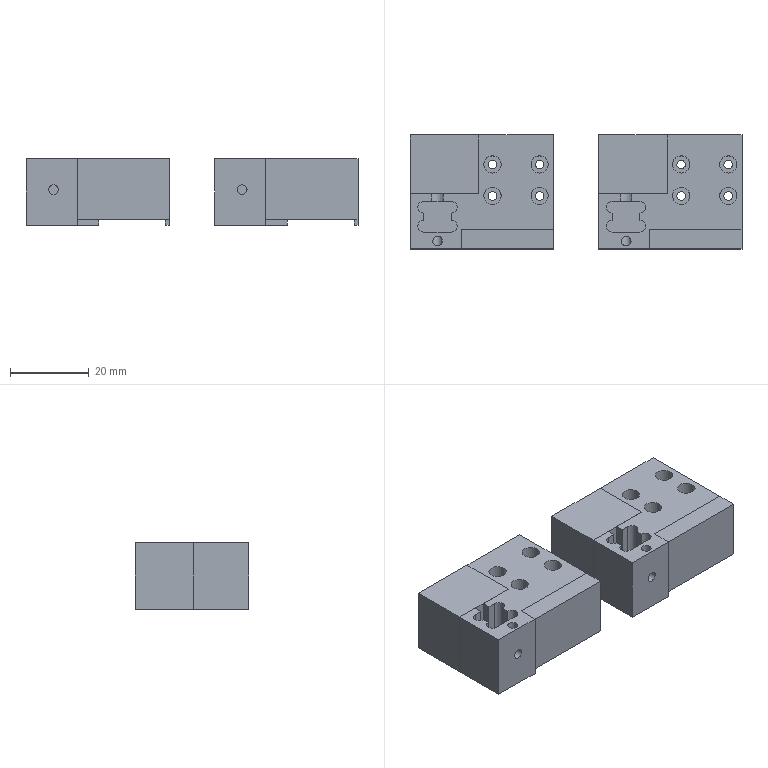NC program | NX | posted with a generic post | part box 84.5 x 29 x 17 mm
Lines 1 to 1070 of 5162:
N10 G17 G21 G94 G90
(FLOOR_WALL , TOOL : D63)
N12 T01 M6
N14 G54
N16 G17 G0 G90 X-81.75 Y0. B0. C0. S6500 M3
N18 G43 Z30. H1
N20 Z3.
N22 G94 G1 Z0. F1500.
N24 X-78.75
N26 X78.75
N28 X81.75
N30 Z3.
N32 G0 Z30.
N34 M5
(ZLEVEL_PROFILE_1 , TOOL : D10)
N36 T10 M6
N38 G54
N40 G17 G0 G90 X-39.617 Y-19.6 B0. C0. S9500 M3
N42 G43 Z30. H10
N44 Z1.5
N46 G94 G1 X-42.804 Z1.333 F1000.
N48 X-44.148 Y-19.266 Z1.26
N50 X-45.354 Y-18.584 Z1.188
N52 X-46.334 Y-17.604 Z1.115
N54 X-47.016 Y-16.398 Z1.043
N56 X-47.35 Y-15.054 Z0.97
N58 Y-14.5 Z0.941
N60 Y14.5 Z-0.579
N62 Y15.054 Z-0.608
N64 X-47.016 Y16.398 Z-0.681
N66 X-46.334 Y17.604 Z-0.753
N68 X-45.354 Y18.584 Z-0.826
N70 X-44.148 Y19.266 Z-0.898
N72 X-42.804 Y19.6 Z-0.971
N74 X-42.25 Z-1.
N76 X-5.75 F3000.
N78 G2 X-0.65 Y14.5 R5.1
N80 G1 Y-14.5
N82 G2 X-5.75 Y-19.6 R5.1
N84 G1 X-42.25
N86 G2 X-47.35 Y-14.5 R5.1
N88 G1 Y14.5
N90 G2 X-42.25 Y19.6 R5.1
N92 G1 X-5.863 Z-1.635
N94 X-5.476 Y19.593 Z-1.642
N96 X-5.091 Y19.557 Z-1.649
N98 X-4.709 Y19.493 Z-1.655
N100 X-4.334 Y19.399 Z-1.662
N102 X-3.966 Y19.278 Z-1.669
N104 X-3.609 Y19.129 Z-1.676
N106 X-3.264 Y18.953 Z-1.682
N108 X-2.934 Y18.752 Z-1.689
N110 X-2.619 Y18.526 Z-1.696
N112 X-2.323 Y18.277 Z-1.703
N114 X-2.047 Y18.006 Z-1.709
N116 X-1.791 Y17.715 Z-1.716
N118 X-1.559 Y17.406 Z-1.723
N120 X-1.351 Y17.08 Z-1.73
N122 X-1.168 Y16.739 Z-1.736
N124 X-1.011 Y16.385 Z-1.743
N126 X-0.882 Y16.02 Z-1.75
N128 X-0.781 Y15.647 Z-1.757
N130 X-0.708 Y15.266 Z-1.764
N132 X-0.664 Y14.882 Z-1.77
N134 X-0.65 Y14.495 Z-1.777
N136 Y14.108 Z-1.784
N138 Y1.721 Z-2.
N140 Y-14.5
N142 G2 X-5.75 Y-19.6 R5.1
N144 G1 X-42.25
N146 G2 X-47.35 Y-14.5 R5.1
N148 G1 Y14.5
N150 G2 X-42.25 Y19.6 R5.1
N152 G1 X-5.863 Z-2.635
N154 X-5.476 Y19.593 Z-2.642
N156 X-5.091 Y19.557 Z-2.649
N158 X-4.709 Y19.493 Z-2.655
N160 X-4.334 Y19.399 Z-2.662
N162 X-3.966 Y19.278 Z-2.669
N164 X-3.609 Y19.129 Z-2.676
N166 X-3.264 Y18.953 Z-2.682
N168 X-2.934 Y18.752 Z-2.689
N170 X-2.619 Y18.526 Z-2.696
N172 X-2.323 Y18.277 Z-2.703
N174 X-2.047 Y18.006 Z-2.709
N176 X-1.791 Y17.715 Z-2.716
N178 X-1.559 Y17.406 Z-2.723
N180 X-1.351 Y17.08 Z-2.73
N182 X-1.168 Y16.739 Z-2.736
N184 X-1.011 Y16.385 Z-2.743
N186 X-0.882 Y16.02 Z-2.75
N188 X-0.781 Y15.647 Z-2.757
N190 X-0.708 Y15.266 Z-2.764
N192 X-0.664 Y14.882 Z-2.77
N194 X-0.65 Y14.495 Z-2.777
N196 Y14.108 Z-2.784
N198 Y1.721 Z-3.
N200 Y-14.5
N202 G2 X-5.75 Y-19.6 R5.1
N204 G1 X-42.25
N206 G2 X-47.35 Y-14.5 R5.1
N208 G1 Y14.5
N210 G2 X-42.25 Y19.6 R5.1
N212 G1 X-5.863 Z-3.635
N214 X-5.476 Y19.593 Z-3.642
N216 X-5.091 Y19.557 Z-3.649
N218 X-4.709 Y19.493 Z-3.655
N220 X-4.334 Y19.399 Z-3.662
N222 X-3.966 Y19.278 Z-3.669
N224 X-3.609 Y19.129 Z-3.676
N226 X-3.264 Y18.953 Z-3.682
N228 X-2.934 Y18.752 Z-3.689
N230 X-2.619 Y18.526 Z-3.696
N232 X-2.323 Y18.277 Z-3.703
N234 X-2.047 Y18.006 Z-3.709
N236 X-1.791 Y17.715 Z-3.716
N238 X-1.559 Y17.406 Z-3.723
N240 X-1.351 Y17.08 Z-3.73
N242 X-1.168 Y16.739 Z-3.736
N244 X-1.011 Y16.385 Z-3.743
N246 X-0.882 Y16.02 Z-3.75
N248 X-0.781 Y15.647 Z-3.757
N250 X-0.708 Y15.266 Z-3.764
N252 X-0.664 Y14.882 Z-3.77
N254 X-0.65 Y14.495 Z-3.777
N256 Y14.108 Z-3.784
N258 Y1.721 Z-4.
N260 Y-14.5
N262 G2 X-5.75 Y-19.6 R5.1
N264 G1 X-42.25
N266 G2 X-47.35 Y-14.5 R5.1
N268 G1 Y14.5
N270 G2 X-42.25 Y19.6 R5.1
N272 G1 X-5.863 Z-4.635
N274 X-5.476 Y19.593 Z-4.642
N276 X-5.091 Y19.557 Z-4.649
N278 X-4.709 Y19.493 Z-4.655
N280 X-4.334 Y19.399 Z-4.662
N282 X-3.966 Y19.278 Z-4.669
N284 X-3.609 Y19.129 Z-4.676
N286 X-3.264 Y18.953 Z-4.682
N288 X-2.934 Y18.752 Z-4.689
N290 X-2.619 Y18.526 Z-4.696
N292 X-2.323 Y18.277 Z-4.703
N294 X-2.047 Y18.006 Z-4.709
N296 X-1.791 Y17.715 Z-4.716
N298 X-1.559 Y17.406 Z-4.723
N300 X-1.351 Y17.08 Z-4.73
N302 X-1.168 Y16.739 Z-4.736
N304 X-1.011 Y16.385 Z-4.743
N306 X-0.882 Y16.02 Z-4.75
N308 X-0.781 Y15.647 Z-4.757
N310 X-0.708 Y15.266 Z-4.764
N312 X-0.664 Y14.882 Z-4.77
N314 X-0.65 Y14.495 Z-4.777
N316 Y14.108 Z-4.784
N318 Y1.721 Z-5.
N320 Y-14.5
N322 G2 X-5.75 Y-19.6 R5.1
N324 G1 X-42.25
N326 G2 X-47.35 Y-14.5 R5.1
N328 G1 Y14.5
N330 G2 X-42.25 Y19.6 R5.1
N332 G1 X-5.863 Z-5.635
N334 X-5.476 Y19.593 Z-5.642
N336 X-5.091 Y19.557 Z-5.649
N338 X-4.709 Y19.493 Z-5.655
N340 X-4.334 Y19.399 Z-5.662
N342 X-3.966 Y19.278 Z-5.669
N344 X-3.609 Y19.129 Z-5.676
N346 X-3.264 Y18.953 Z-5.682
N348 X-2.934 Y18.752 Z-5.689
N350 X-2.619 Y18.526 Z-5.696
N352 X-2.323 Y18.277 Z-5.703
N354 X-2.047 Y18.006 Z-5.709
N356 X-1.791 Y17.715 Z-5.716
N358 X-1.559 Y17.406 Z-5.723
N360 X-1.351 Y17.08 Z-5.73
N362 X-1.168 Y16.739 Z-5.736
N364 X-1.011 Y16.385 Z-5.743
N366 X-0.882 Y16.02 Z-5.75
N368 X-0.781 Y15.647 Z-5.757
N370 X-0.708 Y15.266 Z-5.764
N372 X-0.664 Y14.882 Z-5.77
N374 X-0.65 Y14.495 Z-5.777
N376 Y14.108 Z-5.784
N378 Y1.721 Z-6.
N380 Y-14.5
N382 G2 X-5.75 Y-19.6 R5.1
N384 G1 X-42.25
N386 G2 X-47.35 Y-14.5 R5.1
N388 G1 Y14.5
N390 G2 X-42.25 Y19.6 R5.1
N392 G1 X-5.863 Z-6.635
N394 X-5.476 Y19.593 Z-6.642
N396 X-5.091 Y19.557 Z-6.649
N398 X-4.709 Y19.493 Z-6.655
N400 X-4.334 Y19.399 Z-6.662
N402 X-3.966 Y19.278 Z-6.669
N404 X-3.609 Y19.129 Z-6.676
N406 X-3.264 Y18.953 Z-6.682
N408 X-2.934 Y18.752 Z-6.689
N410 X-2.619 Y18.526 Z-6.696
N412 X-2.323 Y18.277 Z-6.703
N414 X-2.047 Y18.006 Z-6.709
N416 X-1.791 Y17.715 Z-6.716
N418 X-1.559 Y17.406 Z-6.723
N420 X-1.351 Y17.08 Z-6.73
N422 X-1.168 Y16.739 Z-6.736
N424 X-1.011 Y16.385 Z-6.743
N426 X-0.882 Y16.02 Z-6.75
N428 X-0.781 Y15.647 Z-6.757
N430 X-0.708 Y15.266 Z-6.764
N432 X-0.664 Y14.882 Z-6.77
N434 X-0.65 Y14.495 Z-6.777
N436 Y14.108 Z-6.784
N438 Y1.721 Z-7.
N440 Y-14.5
N442 G2 X-5.75 Y-19.6 R5.1
N444 G1 X-42.25
N446 G2 X-47.35 Y-14.5 R5.1
N448 G1 Y14.5
N450 G2 X-42.25 Y19.6 R5.1
N452 G1 X-5.863 Z-7.635
N454 X-5.476 Y19.593 Z-7.642
N456 X-5.091 Y19.557 Z-7.649
N458 X-4.709 Y19.493 Z-7.655
N460 X-4.334 Y19.399 Z-7.662
N462 X-3.966 Y19.278 Z-7.669
N464 X-3.609 Y19.129 Z-7.676
N466 X-3.264 Y18.953 Z-7.682
N468 X-2.934 Y18.752 Z-7.689
N470 X-2.619 Y18.526 Z-7.696
N472 X-2.323 Y18.277 Z-7.703
N474 X-2.047 Y18.006 Z-7.709
N476 X-1.791 Y17.715 Z-7.716
N478 X-1.559 Y17.406 Z-7.723
N480 X-1.351 Y17.08 Z-7.73
N482 X-1.168 Y16.739 Z-7.736
N484 X-1.011 Y16.385 Z-7.743
N486 X-0.882 Y16.02 Z-7.75
N488 X-0.781 Y15.647 Z-7.757
N490 X-0.708 Y15.266 Z-7.764
N492 X-0.664 Y14.882 Z-7.77
N494 X-0.65 Y14.495 Z-7.777
N496 Y14.108 Z-7.784
N498 Y1.721 Z-8.
N500 Y-14.5
N502 G2 X-5.75 Y-19.6 R5.1
N504 G1 X-42.25
N506 G2 X-47.35 Y-14.5 R5.1
N508 G1 Y14.5
N510 G2 X-42.25 Y19.6 R5.1
N512 G1 X-5.863 Z-8.635
N514 X-5.476 Y19.593 Z-8.642
N516 X-5.091 Y19.557 Z-8.649
N518 X-4.709 Y19.493 Z-8.655
N520 X-4.334 Y19.399 Z-8.662
N522 X-3.966 Y19.278 Z-8.669
N524 X-3.609 Y19.129 Z-8.676
N526 X-3.264 Y18.953 Z-8.682
N528 X-2.934 Y18.752 Z-8.689
N530 X-2.619 Y18.526 Z-8.696
N532 X-2.323 Y18.277 Z-8.703
N534 X-2.047 Y18.006 Z-8.709
N536 X-1.791 Y17.715 Z-8.716
N538 X-1.559 Y17.406 Z-8.723
N540 X-1.351 Y17.08 Z-8.73
N542 X-1.168 Y16.739 Z-8.736
N544 X-1.011 Y16.385 Z-8.743
N546 X-0.882 Y16.02 Z-8.75
N548 X-0.781 Y15.647 Z-8.757
N550 X-0.708 Y15.266 Z-8.764
N552 X-0.664 Y14.882 Z-8.77
N554 X-0.65 Y14.495 Z-8.777
N556 Y14.108 Z-8.784
N558 Y1.721 Z-9.
N560 Y-14.5
N562 G2 X-5.75 Y-19.6 R5.1
N564 G1 X-42.25
N566 G2 X-47.35 Y-14.5 R5.1
N568 G1 Y14.5
N570 G2 X-42.25 Y19.6 R5.1
N572 G1 X-5.863 Z-9.635
N574 X-5.476 Y19.593 Z-9.642
N576 X-5.091 Y19.557 Z-9.649
N578 X-4.709 Y19.493 Z-9.655
N580 X-4.334 Y19.399 Z-9.662
N582 X-3.966 Y19.278 Z-9.669
N584 X-3.609 Y19.129 Z-9.676
N586 X-3.264 Y18.953 Z-9.682
N588 X-2.934 Y18.752 Z-9.689
N590 X-2.619 Y18.526 Z-9.696
N592 X-2.323 Y18.277 Z-9.703
N594 X-2.047 Y18.006 Z-9.709
N596 X-1.791 Y17.715 Z-9.716
N598 X-1.559 Y17.406 Z-9.723
N600 X-1.351 Y17.08 Z-9.73
N602 X-1.168 Y16.739 Z-9.736
N604 X-1.011 Y16.385 Z-9.743
N606 X-0.882 Y16.02 Z-9.75
N608 X-0.781 Y15.647 Z-9.757
N610 X-0.708 Y15.266 Z-9.764
N612 X-0.664 Y14.882 Z-9.77
N614 X-0.65 Y14.495 Z-9.777
N616 Y14.108 Z-9.784
N618 Y1.721 Z-10.
N620 Y-14.5
N622 G2 X-5.75 Y-19.6 R5.1
N624 G1 X-42.25
N626 G2 X-47.35 Y-14.5 R5.1
N628 G1 Y14.5
N630 G2 X-42.25 Y19.6 R5.1
N632 G1 X-5.863 Z-10.635
N634 X-5.476 Y19.593 Z-10.642
N636 X-5.091 Y19.557 Z-10.649
N638 X-4.709 Y19.493 Z-10.655
N640 X-4.334 Y19.399 Z-10.662
N642 X-3.966 Y19.278 Z-10.669
N644 X-3.609 Y19.129 Z-10.676
N646 X-3.264 Y18.953 Z-10.682
N648 X-2.934 Y18.752 Z-10.689
N650 X-2.619 Y18.526 Z-10.696
N652 X-2.323 Y18.277 Z-10.703
N654 X-2.047 Y18.006 Z-10.709
N656 X-1.791 Y17.715 Z-10.716
N658 X-1.559 Y17.406 Z-10.723
N660 X-1.351 Y17.08 Z-10.73
N662 X-1.168 Y16.739 Z-10.736
N664 X-1.011 Y16.385 Z-10.743
N666 X-0.882 Y16.02 Z-10.75
N668 X-0.781 Y15.647 Z-10.757
N670 X-0.708 Y15.266 Z-10.764
N672 X-0.664 Y14.882 Z-10.77
N674 X-0.65 Y14.495 Z-10.777
N676 Y14.108 Z-10.784
N678 Y1.721 Z-11.
N680 Y-14.5
N682 G2 X-5.75 Y-19.6 R5.1
N684 G1 X-42.25
N686 G2 X-47.35 Y-14.5 R5.1
N688 G1 Y14.5
N690 G2 X-42.25 Y19.6 R5.1
N692 G1 X-5.863 Z-11.635
N694 X-5.476 Y19.593 Z-11.642
N696 X-5.091 Y19.557 Z-11.649
N698 X-4.709 Y19.493 Z-11.655
N700 X-4.334 Y19.399 Z-11.662
N702 X-3.966 Y19.278 Z-11.669
N704 X-3.609 Y19.129 Z-11.676
N706 X-3.264 Y18.953 Z-11.682
N708 X-2.934 Y18.752 Z-11.689
N710 X-2.619 Y18.526 Z-11.696
N712 X-2.323 Y18.277 Z-11.703
N714 X-2.047 Y18.006 Z-11.709
N716 X-1.791 Y17.715 Z-11.716
N718 X-1.559 Y17.406 Z-11.723
N720 X-1.351 Y17.08 Z-11.73
N722 X-1.168 Y16.739 Z-11.736
N724 X-1.011 Y16.385 Z-11.743
N726 X-0.882 Y16.02 Z-11.75
N728 X-0.781 Y15.647 Z-11.757
N730 X-0.708 Y15.266 Z-11.764
N732 X-0.664 Y14.882 Z-11.77
N734 X-0.65 Y14.495 Z-11.777
N736 Y14.108 Z-11.784
N738 Y1.721 Z-12.
N740 Y-14.5
N742 G2 X-5.75 Y-19.6 R5.1
N744 G1 X-42.25
N746 G2 X-47.35 Y-14.5 R5.1
N748 G1 Y14.5
N750 G2 X-42.25 Y19.6 R5.1
N752 G1 X-5.863 Z-12.635
N754 X-5.476 Y19.593 Z-12.642
N756 X-5.091 Y19.557 Z-12.649
N758 X-4.709 Y19.493 Z-12.655
N760 X-4.334 Y19.399 Z-12.662
N762 X-3.966 Y19.278 Z-12.669
N764 X-3.609 Y19.129 Z-12.676
N766 X-3.264 Y18.953 Z-12.682
N768 X-2.934 Y18.752 Z-12.689
N770 X-2.619 Y18.526 Z-12.696
N772 X-2.323 Y18.277 Z-12.703
N774 X-2.047 Y18.006 Z-12.709
N776 X-1.791 Y17.715 Z-12.716
N778 X-1.559 Y17.406 Z-12.723
N780 X-1.351 Y17.08 Z-12.73
N782 X-1.168 Y16.739 Z-12.736
N784 X-1.011 Y16.385 Z-12.743
N786 X-0.882 Y16.02 Z-12.75
N788 X-0.781 Y15.647 Z-12.757
N790 X-0.708 Y15.266 Z-12.764
N792 X-0.664 Y14.882 Z-12.77
N794 X-0.65 Y14.495 Z-12.777
N796 Y14.108 Z-12.784
N798 Y1.721 Z-13.
N800 Y-14.5
N802 G2 X-5.75 Y-19.6 R5.1
N804 G1 X-42.25
N806 G2 X-47.35 Y-14.5 R5.1
N808 G1 Y14.5
N810 G2 X-42.25 Y19.6 R5.1
N812 G1 X-5.863 Z-13.635
N814 X-5.476 Y19.593 Z-13.642
N816 X-5.091 Y19.557 Z-13.649
N818 X-4.709 Y19.493 Z-13.655
N820 X-4.334 Y19.399 Z-13.662
N822 X-3.966 Y19.278 Z-13.669
N824 X-3.609 Y19.129 Z-13.676
N826 X-3.264 Y18.953 Z-13.682
N828 X-2.934 Y18.752 Z-13.689
N830 X-2.619 Y18.526 Z-13.696
N832 X-2.323 Y18.277 Z-13.703
N834 X-2.047 Y18.006 Z-13.709
N836 X-1.791 Y17.715 Z-13.716
N838 X-1.559 Y17.406 Z-13.723
N840 X-1.351 Y17.08 Z-13.73
N842 X-1.168 Y16.739 Z-13.736
N844 X-1.011 Y16.385 Z-13.743
N846 X-0.882 Y16.02 Z-13.75
N848 X-0.781 Y15.647 Z-13.757
N850 X-0.708 Y15.266 Z-13.764
N852 X-0.664 Y14.882 Z-13.77
N854 X-0.65 Y14.495 Z-13.777
N856 Y14.108 Z-13.784
N858 Y1.721 Z-14.
N860 Y-14.5
N862 G2 X-5.75 Y-19.6 R5.1
N864 G1 X-42.25
N866 G2 X-47.35 Y-14.5 R5.1
N868 G1 Y14.5
N870 G2 X-42.25 Y19.6 R5.1
N872 G1 X-5.863 Z-14.635
N874 X-5.476 Y19.593 Z-14.642
N876 X-5.091 Y19.557 Z-14.649
N878 X-4.709 Y19.493 Z-14.655
N880 X-4.334 Y19.399 Z-14.662
N882 X-3.966 Y19.278 Z-14.669
N884 X-3.609 Y19.129 Z-14.676
N886 X-3.264 Y18.953 Z-14.682
N888 X-2.934 Y18.752 Z-14.689
N890 X-2.619 Y18.526 Z-14.696
N892 X-2.323 Y18.277 Z-14.703
N894 X-2.047 Y18.006 Z-14.709
N896 X-1.791 Y17.715 Z-14.716
N898 X-1.559 Y17.406 Z-14.723
N900 X-1.351 Y17.08 Z-14.73
N902 X-1.168 Y16.739 Z-14.736
N904 X-1.011 Y16.385 Z-14.743
N906 X-0.882 Y16.02 Z-14.75
N908 X-0.781 Y15.647 Z-14.757
N910 X-0.708 Y15.266 Z-14.764
N912 X-0.664 Y14.882 Z-14.77
N914 X-0.65 Y14.495 Z-14.777
N916 Y14.108 Z-14.784
N918 Y1.721 Z-15.
N920 Y-14.5
N922 G2 X-5.75 Y-19.6 R5.1
N924 G1 X-42.25
N926 G2 X-47.35 Y-14.5 R5.1
N928 G1 Y14.5
N930 G2 X-42.25 Y19.6 R5.1
N932 G1 X-5.863 Z-15.635
N934 X-5.476 Y19.593 Z-15.642
N936 X-5.091 Y19.557 Z-15.649
N938 X-4.709 Y19.493 Z-15.655
N940 X-4.334 Y19.399 Z-15.662
N942 X-3.966 Y19.278 Z-15.669
N944 X-3.609 Y19.129 Z-15.676
N946 X-3.264 Y18.953 Z-15.682
N948 X-2.934 Y18.752 Z-15.689
N950 X-2.619 Y18.526 Z-15.696
N952 X-2.323 Y18.277 Z-15.703
N954 X-2.047 Y18.006 Z-15.709
N956 X-1.791 Y17.715 Z-15.716
N958 X-1.559 Y17.406 Z-15.723
N960 X-1.351 Y17.08 Z-15.73
N962 X-1.168 Y16.739 Z-15.736
N964 X-1.011 Y16.385 Z-15.743
N966 X-0.882 Y16.02 Z-15.75
N968 X-0.781 Y15.647 Z-15.757
N970 X-0.708 Y15.266 Z-15.764
N972 X-0.664 Y14.882 Z-15.77
N974 X-0.65 Y14.495 Z-15.777
N976 Y14.108 Z-15.784
N978 Y1.721 Z-16.
N980 Y-14.5
N982 G2 X-5.75 Y-19.6 R5.1
N984 G1 X-42.25
N986 G2 X-47.35 Y-14.5 R5.1
N988 G1 Y14.5
N990 G2 X-42.25 Y19.6 R5.1
N992 G1 X-5.863 Z-16.635
N994 X-5.476 Y19.593 Z-16.642
N996 X-5.091 Y19.557 Z-16.649
N998 X-4.709 Y19.493 Z-16.655
N1000 X-4.334 Y19.399 Z-16.662
N1002 X-3.966 Y19.278 Z-16.669
N1004 X-3.609 Y19.129 Z-16.676
N1006 X-3.264 Y18.953 Z-16.682
N1008 X-2.934 Y18.752 Z-16.689
N1010 X-2.619 Y18.526 Z-16.696
N1012 X-2.323 Y18.277 Z-16.703
N1014 X-2.047 Y18.006 Z-16.709
N1016 X-1.791 Y17.715 Z-16.716
N1018 X-1.559 Y17.406 Z-16.723
N1020 X-1.351 Y17.08 Z-16.73
N1022 X-1.168 Y16.739 Z-16.736
N1024 X-1.011 Y16.385 Z-16.743
N1026 X-0.882 Y16.02 Z-16.75
N1028 X-0.781 Y15.647 Z-16.757
N1030 X-0.708 Y15.266 Z-16.764
N1032 X-0.664 Y14.882 Z-16.77
N1034 X-0.65 Y14.495 Z-16.777
N1036 Y14.108 Z-16.784
N1038 Y1.721 Z-17.
N1040 Y-14.5
N1042 G2 X-5.75 Y-19.6 R5.1
N1044 G1 X-42.25
N1046 G2 X-47.35 Y-14.5 R5.1
N1048 G1 Y14.5
N1050 G2 X-42.25 Y19.6 R5.1
N1052 G1 X-5.75
N1054 G2 X-0.65 Y14.5 R5.1
N1056 G1 Y1.721
N1058 Z-15.5
N1060 G0 Z30.
N1062 X8.383 Y-19.6
N1064 Z1.5
N1066 G1 X5.196 Z1.333 F1000.
N1068 X3.852 Y-19.266 Z1.26
N1070 X2.646 Y-18.584 Z1.188
N1072 X1.666 Y-17.604 Z1.115
N1074 X0.984 Y-16.398 Z1.043
N1076 X0.65 Y-15.054 Z0.97
N1078 Y15.054 Z-0.608
N1080 X0.984 Y16.398 Z-0.681
N1082 X1.666 Y17.604 Z-0.753
N1084 X2.646 Y18.584 Z-0.826
N1086 X3.852 Y19.266 Z-0.898
N1088 X5.196 Y19.6 Z-0.971
N1090 X5.75 Z-1.
N1092 X42.25 F3000.
N1094 G2 X47.35 Y14.5 R5.1
N1096 G1 Y-14.5
N1098 G2 X42.25 Y-19.6 R5.1
N1100 G1 X5.75
N1102 G2 X0.65 Y-14.5 R5.1
N1104 G1 Y14.5
N1106 G2 X5.75 Y19.6 R5.1
N1108 G1 X42.137 Z-1.635
N1110 X42.524 Y19.593 Z-1.642
N1112 X42.909 Y19.557 Z-1.649
N1114 X43.291 Y19.493 Z-1.655
N1116 X43.666 Y19.399 Z-1.662
N1118 X44.034 Y19.278 Z-1.669
N1120 X44.391 Y19.129 Z-1.676
N1122 X44.736 Y18.953 Z-1.682
N1124 X45.066 Y18.752 Z-1.689
N1126 X45.381 Y18.526 Z-1.696
N1128 X45.677 Y18.277 Z-1.703
N1130 X45.953 Y18.006 Z-1.709
N1132 X46.209 Y17.715 Z-1.716
N1134 X46.441 Y17.406 Z-1.723
N1136 X46.649 Y17.08 Z-1.73
N1138 X46.832 Y16.739 Z-1.736
N1140 X46.989 Y16.385 Z-1.743
N1142 X47.118 Y16.02 Z-1.75
N1144 X47.219 Y15.647 Z-1.757
N1146 X47.292 Y15.266 Z-1.764
N1148 X47.336 Y14.882 Z-1.77
N1150 X47.35 Y14.495 Z-1.777
N1152 Y14.108 Z-1.784
N1154 Y1.721 Z-2.
N1156 Y-14.5
N1158 G2 X42.25 Y-19.6 R5.1
N1160 G1 X5.75
N1162 G2 X0.65 Y-14.5 R5.1
N1164 G1 Y14.5
N1166 G2 X5.75 Y19.6 R5.1
N1168 G1 X42.137 Z-2.635
N1170 X42.524 Y19.593 Z-2.642
N1172 X42.909 Y19.557 Z-2.649
N1174 X43.291 Y19.493 Z-2.655
N1176 X43.666 Y19.399 Z-2.662
N1178 X44.034 Y19.278 Z-2.669
N1180 X44.391 Y19.129 Z-2.676
N1182 X44.736 Y18.953 Z-2.682
N1184 X45.066 Y18.752 Z-2.689
N1186 X45.381 Y18.526 Z-2.696
N1188 X45.677 Y18.277 Z-2.703
N1190 X45.953 Y18.006 Z-2.709
N1192 X46.209 Y17.715 Z-2.716
N1194 X46.441 Y17.406 Z-2.723
N1196 X46.649 Y17.08 Z-2.73
N1198 X46.832 Y16.739 Z-2.736
N1200 X46.989 Y16.385 Z-2.743
N1202 X47.118 Y16.02 Z-2.75
N1204 X47.219 Y15.647 Z-2.757
N1206 X47.292 Y15.266 Z-2.764
N1208 X47.336 Y14.882 Z-2.77
N1210 X47.35 Y14.495 Z-2.777
N1212 Y14.108 Z-2.784
N1214 Y1.721 Z-3.
N1216 Y-14.5
N1218 G2 X42.25 Y-19.6 R5.1
N1220 G1 X5.75
N1222 G2 X0.65 Y-14.5 R5.1
N1224 G1 Y14.5
N1226 G2 X5.75 Y19.6 R5.1
N1228 G1 X42.137 Z-3.635
N1230 X42.524 Y19.593 Z-3.642
N1232 X42.909 Y19.557 Z-3.649
N1234 X43.291 Y19.493 Z-3.655
N1236 X43.666 Y19.399 Z-3.662
N1238 X44.034 Y19.278 Z-3.669
N1240 X44.391 Y19.129 Z-3.676
N1242 X44.736 Y18.953 Z-3.682
N1244 X45.066 Y18.752 Z-3.689
N1246 X45.381 Y18.526 Z-3.696
N1248 X45.677 Y18.277 Z-3.703
N1250 X45.953 Y18.006 Z-3.709
N1252 X46.209 Y17.715 Z-3.716
N1254 X46.441 Y17.406 Z-3.723
N1256 X46.649 Y17.08 Z-3.73
N1258 X46.832 Y16.739 Z-3.736
N1260 X46.989 Y16.385 Z-3.743
N1262 X47.118 Y16.02 Z-3.75
N1264 X47.219 Y15.647 Z-3.757
N1266 X47.292 Y15.266 Z-3.764
N1268 X47.336 Y14.882 Z-3.77
N1270 X47.35 Y14.495 Z-3.777
N1272 Y14.108 Z-3.784
N1274 Y1.721 Z-4.
N1276 Y-14.5
N1278 G2 X42.25 Y-19.6 R5.1
N1280 G1 X5.75
N1282 G2 X0.65 Y-14.5 R5.1
N1284 G1 Y14.5
N1286 G2 X5.75 Y19.6 R5.1
N1288 G1 X42.137 Z-4.635
N1290 X42.524 Y19.593 Z-4.642
N1292 X42.909 Y19.557 Z-4.649
N1294 X43.291 Y19.493 Z-4.655
N1296 X43.666 Y19.399 Z-4.662
N1298 X44.034 Y19.278 Z-4.669
N1300 X44.391 Y19.129 Z-4.676
N1302 X44.736 Y18.953 Z-4.682
N1304 X45.066 Y18.752 Z-4.689
N1306 X45.381 Y18.526 Z-4.696
N1308 X45.677 Y18.277 Z-4.703
N1310 X45.953 Y18.006 Z-4.709
N1312 X46.209 Y17.715 Z-4.716
N1314 X46.441 Y17.406 Z-4.723
N1316 X46.649 Y17.08 Z-4.73
N1318 X46.832 Y16.739 Z-4.736
N1320 X46.989 Y16.385 Z-4.743
N1322 X47.118 Y16.02 Z-4.75
N1324 X47.219 Y15.647 Z-4.757
N1326 X47.292 Y15.266 Z-4.764
N1328 X47.336 Y14.882 Z-4.77
N1330 X47.35 Y14.495 Z-4.777
N1332 Y14.108 Z-4.784
N1334 Y1.721 Z-5.
N1336 Y-14.5
N1338 G2 X42.25 Y-19.6 R5.1
N1340 G1 X5.75
N1342 G2 X0.65 Y-14.5 R5.1
N1344 G1 Y14.5
N1346 G2 X5.75 Y19.6 R5.1
N1348 G1 X42.137 Z-5.635
N1350 X42.524 Y19.593 Z-5.642
N1352 X42.909 Y19.557 Z-5.649
N1354 X43.291 Y19.493 Z-5.655
N1356 X43.666 Y19.399 Z-5.662
N1358 X44.034 Y19.278 Z-5.669
N1360 X44.391 Y19.129 Z-5.676
N1362 X44.736 Y18.953 Z-5.682
N1364 X45.066 Y18.752 Z-5.689
N1366 X45.381 Y18.526 Z-5.696
N1368 X45.677 Y18.277 Z-5.703
N1370 X45.953 Y18.006 Z-5.709
N1372 X46.209 Y17.715 Z-5.716
N1374 X46.441 Y17.406 Z-5.723
N1376 X46.649 Y17.08 Z-5.73
N1378 X46.832 Y16.739 Z-5.736
N1380 X46.989 Y16.385 Z-5.743
N1382 X47.118 Y16.02 Z-5.75
N1384 X47.219 Y15.647 Z-5.757
N1386 X47.292 Y15.266 Z-5.764
N1388 X47.336 Y14.882 Z-5.77
N1390 X47.35 Y14.495 Z-5.777
N1392 Y14.108 Z-5.784
N1394 Y1.721 Z-6.
N1396 Y-14.5
N1398 G2 X42.25 Y-19.6 R5.1
N1400 G1 X5.75
N1402 G2 X0.65 Y-14.5 R5.1
N1404 G1 Y14.5
N1406 G2 X5.75 Y19.6 R5.1
N1408 G1 X42.137 Z-6.635
N1410 X42.524 Y19.593 Z-6.642
N1412 X42.909 Y19.557 Z-6.649
N1414 X43.291 Y19.493 Z-6.655
N1416 X43.666 Y19.399 Z-6.662
N1418 X44.034 Y19.278 Z-6.669
N1420 X44.391 Y19.129 Z-6.676
N1422 X44.736 Y18.953 Z-6.682
N1424 X45.066 Y18.752 Z-6.689
N1426 X45.381 Y18.526 Z-6.696
N1428 X45.677 Y18.277 Z-6.703
N1430 X45.953 Y18.006 Z-6.709
N1432 X46.209 Y17.715 Z-6.716
N1434 X46.441 Y17.406 Z-6.723
N1436 X46.649 Y17.08 Z-6.73
N1438 X46.832 Y16.739 Z-6.736
N1440 X46.989 Y16.385 Z-6.743
N1442 X47.118 Y16.02 Z-6.75
N1444 X47.219 Y15.647 Z-6.757
N1446 X47.292 Y15.266 Z-6.764
N1448 X47.336 Y14.882 Z-6.77
N1450 X47.35 Y14.495 Z-6.777
N1452 Y14.108 Z-6.784
N1454 Y1.721 Z-7.
N1456 Y-14.5
N1458 G2 X42.25 Y-19.6 R5.1
N1460 G1 X5.75
N1462 G2 X0.65 Y-14.5 R5.1
N1464 G1 Y14.5
N1466 G2 X5.75 Y19.6 R5.1
N1468 G1 X42.137 Z-7.635
N1470 X42.524 Y19.593 Z-7.642
N1472 X42.909 Y19.557 Z-7.649
N1474 X43.291 Y19.493 Z-7.655
N1476 X43.666 Y19.399 Z-7.662
N1478 X44.034 Y19.278 Z-7.669
N1480 X44.391 Y19.129 Z-7.676
N1482 X44.736 Y18.953 Z-7.682
N1484 X45.066 Y18.752 Z-7.689
N1486 X45.381 Y18.526 Z-7.696
N1488 X45.677 Y18.277 Z-7.703
N1490 X45.953 Y18.006 Z-7.709
N1492 X46.209 Y17.715 Z-7.716
N1494 X46.441 Y17.406 Z-7.723
N1496 X46.649 Y17.08 Z-7.73
N1498 X46.832 Y16.739 Z-7.736
N1500 X46.989 Y16.385 Z-7.743
N1502 X47.118 Y16.02 Z-7.75
N1504 X47.219 Y15.647 Z-7.757
N1506 X47.292 Y15.266 Z-7.764
N1508 X47.336 Y14.882 Z-7.77
N1510 X47.35 Y14.495 Z-7.777
N1512 Y14.108 Z-7.784
N1514 Y1.721 Z-8.
N1516 Y-14.5
N1518 G2 X42.25 Y-19.6 R5.1
N1520 G1 X5.75
N1522 G2 X0.65 Y-14.5 R5.1
N1524 G1 Y14.5
N1526 G2 X5.75 Y19.6 R5.1
N1528 G1 X42.137 Z-8.635
N1530 X42.524 Y19.593 Z-8.642
N1532 X42.909 Y19.557 Z-8.649
N1534 X43.291 Y19.493 Z-8.655
N1536 X43.666 Y19.399 Z-8.662
N1538 X44.034 Y19.278 Z-8.669
N1540 X44.391 Y19.129 Z-8.676
N1542 X44.736 Y18.953 Z-8.682
N1544 X45.066 Y18.752 Z-8.689
N1546 X45.381 Y18.526 Z-8.696
N1548 X45.677 Y18.277 Z-8.703
N1550 X45.953 Y18.006 Z-8.709
N1552 X46.209 Y17.715 Z-8.716
N1554 X46.441 Y17.406 Z-8.723
N1556 X46.649 Y17.08 Z-8.73
N1558 X46.832 Y16.739 Z-8.736
N1560 X46.989 Y16.385 Z-8.743
N1562 X47.118 Y16.02 Z-8.75
N1564 X47.219 Y15.647 Z-8.757
N1566 X47.292 Y15.266 Z-8.764
N1568 X47.336 Y14.882 Z-8.77
N1570 X47.35 Y14.495 Z-8.777
N1572 Y14.108 Z-8.784
N1574 Y1.721 Z-9.
N1576 Y-14.5
N1578 G2 X42.25 Y-19.6 R5.1
N1580 G1 X5.75
N1582 G2 X0.65 Y-14.5 R5.1
N1584 G1 Y14.5
N1586 G2 X5.75 Y19.6 R5.1
N1588 G1 X42.137 Z-9.635
N1590 X42.524 Y19.593 Z-9.642
N1592 X42.909 Y19.557 Z-9.649
N1594 X43.291 Y19.493 Z-9.655
N1596 X43.666 Y19.399 Z-9.662
N1598 X44.034 Y19.278 Z-9.669
N1600 X44.391 Y19.129 Z-9.676
N1602 X44.736 Y18.953 Z-9.682
N1604 X45.066 Y18.752 Z-9.689
N1606 X45.381 Y18.526 Z-9.696
N1608 X45.677 Y18.277 Z-9.703
N1610 X45.953 Y18.006 Z-9.709
N1612 X46.209 Y17.715 Z-9.716
N1614 X46.441 Y17.406 Z-9.723
N1616 X46.649 Y17.08 Z-9.73
N1618 X46.832 Y16.739 Z-9.736
N1620 X46.989 Y16.385 Z-9.743
N1622 X47.118 Y16.02 Z-9.75
N1624 X47.219 Y15.647 Z-9.757
N1626 X47.292 Y15.266 Z-9.764
N1628 X47.336 Y14.882 Z-9.77
N1630 X47.35 Y14.495 Z-9.777
N1632 Y14.108 Z-9.784
N1634 Y1.721 Z-10.
N1636 Y-14.5
N1638 G2 X42.25 Y-19.6 R5.1
N1640 G1 X5.75
N1642 G2 X0.65 Y-14.5 R5.1
N1644 G1 Y14.5
N1646 G2 X5.75 Y19.6 R5.1
N1648 G1 X42.137 Z-10.635
N1650 X42.524 Y19.593 Z-10.642
N1652 X42.909 Y19.557 Z-10.649
N1654 X43.291 Y19.493 Z-10.655
N1656 X43.666 Y19.399 Z-10.662
N1658 X44.034 Y19.278 Z-10.669
N1660 X44.391 Y19.129 Z-10.676
N1662 X44.736 Y18.953 Z-10.682
N1664 X45.066 Y18.752 Z-10.689
N1666 X45.381 Y18.526 Z-10.696
N1668 X45.677 Y18.277 Z-10.703
N1670 X45.953 Y18.006 Z-10.709
N1672 X46.209 Y17.715 Z-10.716
N1674 X46.441 Y17.406 Z-10.723
N1676 X46.649 Y17.08 Z-10.73
N1678 X46.832 Y16.739 Z-10.736
N1680 X46.989 Y16.385 Z-10.743
N1682 X47.118 Y16.02 Z-10.75
N1684 X47.219 Y15.647 Z-10.757
N1686 X47.292 Y15.266 Z-10.764
N1688 X47.336 Y14.882 Z-10.77
N1690 X47.35 Y14.495 Z-10.777
N1692 Y14.108 Z-10.784
N1694 Y1.721 Z-11.
N1696 Y-14.5
N1698 G2 X42.25 Y-19.6 R5.1
N1700 G1 X5.75
N1702 G2 X0.65 Y-14.5 R5.1
N1704 G1 Y14.5
N1706 G2 X5.75 Y19.6 R5.1
N1708 G1 X42.137 Z-11.635
N1710 X42.524 Y19.593 Z-11.642
N1712 X42.909 Y19.557 Z-11.649
N1714 X43.291 Y19.493 Z-11.655
N1716 X43.666 Y19.399 Z-11.662
N1718 X44.034 Y19.278 Z-11.669
N1720 X44.391 Y19.129 Z-11.676
N1722 X44.736 Y18.953 Z-11.682
N1724 X45.066 Y18.752 Z-11.689
N1726 X45.381 Y18.526 Z-11.696
N1728 X45.677 Y18.277 Z-11.703
N1730 X45.953 Y18.006 Z-11.709
N1732 X46.209 Y17.715 Z-11.716
N1734 X46.441 Y17.406 Z-11.723
N1736 X46.649 Y17.08 Z-11.73
N1738 X46.832 Y16.739 Z-11.736
N1740 X46.989 Y16.385 Z-11.743
N1742 X47.118 Y16.02 Z-11.75
N1744 X47.219 Y15.647 Z-11.757
N1746 X47.292 Y15.266 Z-11.764
N1748 X47.336 Y14.882 Z-11.77
N1750 X47.35 Y14.495 Z-11.777
N1752 Y14.108 Z-11.784
N1754 Y1.721 Z-12.
N1756 Y-14.5
N1758 G2 X42.25 Y-19.6 R5.1
N1760 G1 X5.75
N1762 G2 X0.65 Y-14.5 R5.1
N1764 G1 Y14.5
N1766 G2 X5.75 Y19.6 R5.1
N1768 G1 X42.137 Z-12.635
N1770 X42.524 Y19.593 Z-12.642
N1772 X42.909 Y19.557 Z-12.649
N1774 X43.291 Y19.493 Z-12.655
N1776 X43.666 Y19.399 Z-12.662
N1778 X44.034 Y19.278 Z-12.669
N1780 X44.391 Y19.129 Z-12.676
N1782 X44.736 Y18.953 Z-12.682
N1784 X45.066 Y18.752 Z-12.689
N1786 X45.381 Y18.526 Z-12.696
N1788 X45.677 Y18.277 Z-12.703
N1790 X45.953 Y18.006 Z-12.709
N1792 X46.209 Y17.715 Z-12.716
N1794 X46.441 Y17.406 Z-12.723
N1796 X46.649 Y17.08 Z-12.73
N1798 X46.832 Y16.739 Z-12.736
N1800 X46.989 Y16.385 Z-12.743
N1802 X47.118 Y16.02 Z-12.75
N1804 X47.219 Y15.647 Z-12.757
N1806 X47.292 Y15.266 Z-12.764
N1808 X47.336 Y14.882 Z-12.77
N1810 X47.35 Y14.495 Z-12.777
N1812 Y14.108 Z-12.784
N1814 Y1.721 Z-13.
N1816 Y-14.5
N1818 G2 X42.25 Y-19.6 R5.1
N1820 G1 X5.75
N1822 G2 X0.65 Y-14.5 R5.1
N1824 G1 Y14.5
N1826 G2 X5.75 Y19.6 R5.1
N1828 G1 X42.137 Z-13.635
N1830 X42.524 Y19.593 Z-13.642
N1832 X42.909 Y19.557 Z-13.649
N1834 X43.291 Y19.493 Z-13.655
N1836 X43.666 Y19.399 Z-13.662
N1838 X44.034 Y19.278 Z-13.669
N1840 X44.391 Y19.129 Z-13.676
N1842 X44.736 Y18.953 Z-13.682
N1844 X45.066 Y18.752 Z-13.689
N1846 X45.381 Y18.526 Z-13.696
N1848 X45.677 Y18.277 Z-13.703
N1850 X45.953 Y18.006 Z-13.709
N1852 X46.209 Y17.715 Z-13.716
N1854 X46.441 Y17.406 Z-13.723
N1856 X46.649 Y17.08 Z-13.73
N1858 X46.832 Y16.739 Z-13.736
N1860 X46.989 Y16.385 Z-13.743
N1862 X47.118 Y16.02 Z-13.75
N1864 X47.219 Y15.647 Z-13.757
N1866 X47.292 Y15.266 Z-13.764
N1868 X47.336 Y14.882 Z-13.77
N1870 X47.35 Y14.495 Z-13.777
N1872 Y14.108 Z-13.784
N1874 Y1.721 Z-14.
N1876 Y-14.5
N1878 G2 X42.25 Y-19.6 R5.1
N1880 G1 X5.75
N1882 G2 X0.65 Y-14.5 R5.1
N1884 G1 Y14.5
N1886 G2 X5.75 Y19.6 R5.1
N1888 G1 X42.137 Z-14.635
N1890 X42.524 Y19.593 Z-14.642
N1892 X42.909 Y19.557 Z-14.649
N1894 X43.291 Y19.493 Z-14.655
N1896 X43.666 Y19.399 Z-14.662
N1898 X44.034 Y19.278 Z-14.669
N1900 X44.391 Y19.129 Z-14.676
N1902 X44.736 Y18.953 Z-14.682
N1904 X45.066 Y18.752 Z-14.689
N1906 X45.381 Y18.526 Z-14.696
N1908 X45.677 Y18.277 Z-14.703
N1910 X45.953 Y18.006 Z-14.709
N1912 X46.209 Y17.715 Z-14.716
N1914 X46.441 Y17.406 Z-14.723
N1916 X46.649 Y17.08 Z-14.73
N1918 X46.832 Y16.739 Z-14.736
N1920 X46.989 Y16.385 Z-14.743
N1922 X47.118 Y16.02 Z-14.75
N1924 X47.219 Y15.647 Z-14.757
N1926 X47.292 Y15.266 Z-14.764
N1928 X47.336 Y14.882 Z-14.77
N1930 X47.35 Y14.495 Z-14.777
N1932 Y14.108 Z-14.784
N1934 Y1.721 Z-15.
N1936 Y-14.5
N1938 G2 X42.25 Y-19.6 R5.1
N1940 G1 X5.75
N1942 G2 X0.65 Y-14.5 R5.1
N1944 G1 Y14.5
N1946 G2 X5.75 Y19.6 R5.1
N1948 G1 X42.137 Z-15.635
N1950 X42.524 Y19.593 Z-15.642
N1952 X42.909 Y19.557 Z-15.649
N1954 X43.291 Y19.493 Z-15.655
N1956 X43.666 Y19.399 Z-15.662
N1958 X44.034 Y19.278 Z-15.669
N1960 X44.391 Y19.129 Z-15.676
N1962 X44.736 Y18.953 Z-15.682
N1964 X45.066 Y18.752 Z-15.689
N1966 X45.381 Y18.526 Z-15.696
N1968 X45.677 Y18.277 Z-15.703
N1970 X45.953 Y18.006 Z-15.709
N1972 X46.209 Y17.715 Z-15.716
N1974 X46.441 Y17.406 Z-15.723
N1976 X46.649 Y17.08 Z-15.73
N1978 X46.832 Y16.739 Z-15.736
N1980 X46.989 Y16.385 Z-15.743
N1982 X47.118 Y16.02 Z-15.75
N1984 X47.219 Y15.647 Z-15.757
N1986 X47.292 Y15.266 Z-15.764
N1988 X47.336 Y14.882 Z-15.77
N1990 X47.35 Y14.495 Z-15.777
N1992 Y14.108 Z-15.784
N1994 Y1.721 Z-16.
N1996 Y-14.5
N1998 G2 X42.25 Y-19.6 R5.1
N2000 G1 X5.75
N2002 G2 X0.65 Y-14.5 R5.1
N2004 G1 Y14.5
N2006 G2 X5.75 Y19.6 R5.1
N2008 G1 X42.137 Z-16.635
N2010 X42.524 Y19.593 Z-16.642
N2012 X42.909 Y19.557 Z-16.649
N2014 X43.291 Y19.493 Z-16.655
N2016 X43.666 Y19.399 Z-16.662
N2018 X44.034 Y19.278 Z-16.669
N2020 X44.391 Y19.129 Z-16.676
N2022 X44.736 Y18.953 Z-16.682
N2024 X45.066 Y18.752 Z-16.689
N2026 X45.381 Y18.526 Z-16.696
N2028 X45.677 Y18.277 Z-16.703
N2030 X45.953 Y18.006 Z-16.709
N2032 X46.209 Y17.715 Z-16.716
N2034 X46.441 Y17.406 Z-16.723
N2036 X46.649 Y17.08 Z-16.73
N2038 X46.832 Y16.739 Z-16.736
N2040 X46.989 Y16.385 Z-16.743
N2042 X47.118 Y16.02 Z-16.75
N2044 X47.219 Y15.647 Z-16.757
N2046 X47.292 Y15.266 Z-16.764
N2048 X47.336 Y14.882 Z-16.77
N2050 X47.35 Y14.495 Z-16.777
N2052 Y14.108 Z-16.784
N2054 Y1.721 Z-17.
N2056 Y-14.5
N2058 G2 X42.25 Y-19.6 R5.1
N2060 G1 X5.75
N2062 G2 X0.65 Y-14.5 R5.1
N2064 G1 Y14.5
N2066 G2 X5.75 Y19.6 R5.1
N2068 G1 X42.25
N2070 G2 X47.35 Y14.5 R5.1
N2072 G1 Y1.721
N2074 Z-15.5
N2076 G0 Z30.
(DRILLING_COPY , TOOL : 2.5ZT)
N2078 T12 M6
N2080 G17 G43 G0 G90 X-35.25 Y-12.5 Z30. B0. C0. S2000 H12 M3
N2082 G94 G83 G98 Z-10.151 F120. Q2. R3.
N2084 X12.75
N2086 G80
N2088 G0 X12.75 Y-12.5 Z30.
N2090 M5
(DRILLING_COPY_COPY , TOOL : 2.2ZT)
N2092 T14 M6
N2094 G54
N2096 G17 G0 G90 X38.75 Y6.999 B0. C0. S2000 M3
N2098 G43 Z30. H14
N2100 G94 G83 G98 Z-17.658 F120. Q2. R3.
N2102 Y-1.001
N2104 X26.75
N2106 Y6.999
N2108 X-9.25
N2110 Y-1.001
N2112 X-21.25
N2114 Y6.999
N2116 G80
N2118 G0 X-21.25 Y6.999 Z30.
N2120 M5